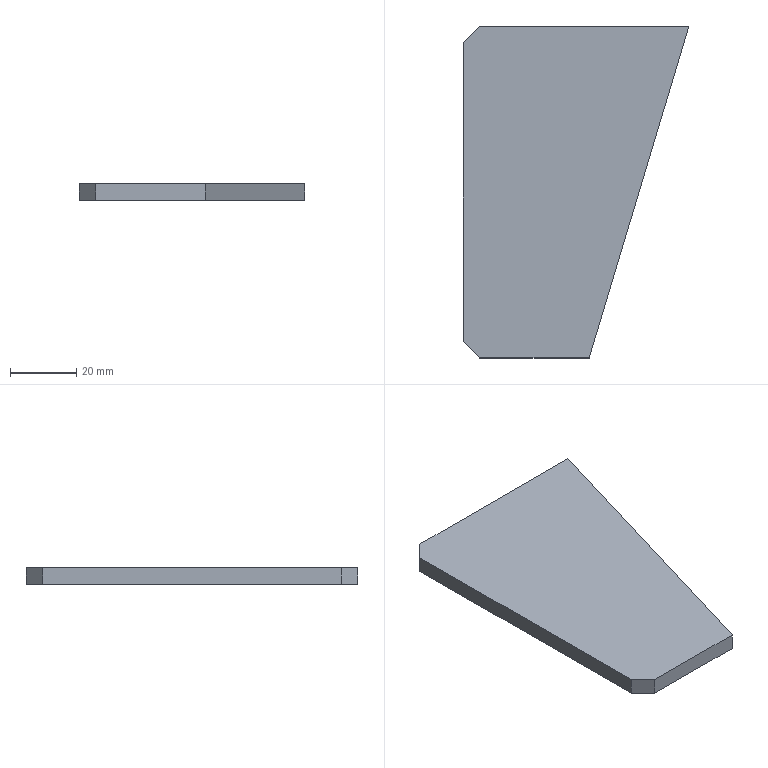Part | STEP file | 750038122 | 1 solid | 8 faces | box 68 x 100 x 5 mm | volume 26375 mm3 | plane 8
STEP:
#1=CARTESIAN_POINT('',(38.,0.,5.));
#2=VERTEX_POINT('',#1);
#3=CARTESIAN_POINT('',(5.,0.,5.));
#4=VERTEX_POINT('',#3);
#5=CARTESIAN_POINT('',(0.,0.,5.));
#6=DIRECTION('',(-1.,0.,0.));
#7=VECTOR('',#6,1000.);
#8=LINE('',#5,#7);
#9=EDGE_CURVE('',#2,#4,#8,.T.);
#10=ORIENTED_EDGE('',*,*,#9,.F.);
#11=CARTESIAN_POINT('',(68.,100.,5.));
#12=VERTEX_POINT('',#11);
#13=CARTESIAN_POINT('',(68.,100.,5.));
#14=DIRECTION('',(-0.2873,-0.9578,0.));
#15=VECTOR('',#14,1000.);
#16=LINE('',#13,#15);
#17=EDGE_CURVE('',#12,#2,#16,.T.);
#18=ORIENTED_EDGE('',*,*,#17,.F.);
#19=CARTESIAN_POINT('',(5.,100.,5.));
#20=VERTEX_POINT('',#19);
#21=CARTESIAN_POINT('',(0.,100.,5.));
#22=DIRECTION('',(1.,0.,0.));
#23=VECTOR('',#22,1000.);
#24=LINE('',#21,#23);
#25=EDGE_CURVE('',#20,#12,#24,.T.);
#26=ORIENTED_EDGE('',*,*,#25,.F.);
#27=CARTESIAN_POINT('',(0.,95.,5.));
#28=VERTEX_POINT('',#27);
#29=CARTESIAN_POINT('',(0.,95.,5.));
#30=DIRECTION('',(0.7071,0.7071,0.));
#31=VECTOR('',#30,1000.);
#32=LINE('',#29,#31);
#33=EDGE_CURVE('',#28,#20,#32,.T.);
#34=ORIENTED_EDGE('',*,*,#33,.F.);
#35=CARTESIAN_POINT('',(0.,5.,5.));
#36=VERTEX_POINT('',#35);
#37=CARTESIAN_POINT('',(0.,0.,5.));
#38=DIRECTION('',(0.,1.,0.));
#39=VECTOR('',#38,1000.);
#40=LINE('',#37,#39);
#41=EDGE_CURVE('',#36,#28,#40,.T.);
#42=ORIENTED_EDGE('',*,*,#41,.F.);
#43=CARTESIAN_POINT('',(5.,0.,5.));
#44=DIRECTION('',(-0.7071,0.7071,0.));
#45=VECTOR('',#44,1000.);
#46=LINE('',#43,#45);
#47=EDGE_CURVE('',#4,#36,#46,.T.);
#48=ORIENTED_EDGE('',*,*,#47,.F.);
#49=EDGE_LOOP('',(#10,#18,#26,#34,#42,#48));
#50=FACE_OUTER_BOUND('',#49,.T.);
#51=CARTESIAN_POINT('',(0.,0.,5.));
#52=DIRECTION('',(0.,0.,-1.));
#53=DIRECTION('',(-1.,0.,0.));
#54=AXIS2_PLACEMENT_3D('',#51,#52,#53);
#55=PLANE('',#54);
#56=ADVANCED_FACE('',(#50),#55,.F.);
#57=ORIENTED_EDGE('',*,*,#47,.T.);
#58=CARTESIAN_POINT('',(0.,5.,0.));
#59=VERTEX_POINT('',#58);
#60=CARTESIAN_POINT('',(0.,5.,5.));
#61=DIRECTION('',(0.,0.,-1.));
#62=VECTOR('',#61,1000.);
#63=LINE('',#60,#62);
#64=EDGE_CURVE('',#36,#59,#63,.T.);
#65=ORIENTED_EDGE('',*,*,#64,.T.);
#66=CARTESIAN_POINT('',(5.,0.,0.));
#67=VERTEX_POINT('',#66);
#68=CARTESIAN_POINT('',(5.,0.,0.));
#69=DIRECTION('',(0.7071,-0.7071,0.));
#70=VECTOR('',#69,1000.);
#71=LINE('',#68,#70);
#72=EDGE_CURVE('',#59,#67,#71,.T.);
#73=ORIENTED_EDGE('',*,*,#72,.T.);
#74=CARTESIAN_POINT('',(5.,0.,5.));
#75=DIRECTION('',(0.,0.,1.));
#76=VECTOR('',#75,1000.);
#77=LINE('',#74,#76);
#78=EDGE_CURVE('',#67,#4,#77,.T.);
#79=ORIENTED_EDGE('',*,*,#78,.T.);
#80=EDGE_LOOP('',(#57,#65,#73,#79));
#81=FACE_OUTER_BOUND('',#80,.T.);
#82=CARTESIAN_POINT('',(5.,0.,5.));
#83=DIRECTION('',(-0.7071,-0.7071,0.));
#84=DIRECTION('',(0.7071,-0.7071,0.));
#85=AXIS2_PLACEMENT_3D('',#82,#83,#84);
#86=PLANE('',#85);
#87=ADVANCED_FACE('',(#81),#86,.T.);
#88=ORIENTED_EDGE('',*,*,#9,.T.);
#89=ORIENTED_EDGE('',*,*,#78,.F.);
#90=CARTESIAN_POINT('',(38.,0.,0.));
#91=VERTEX_POINT('',#90);
#92=CARTESIAN_POINT('',(38.,0.,0.));
#93=DIRECTION('',(1.,0.,0.));
#94=VECTOR('',#93,1000.);
#95=LINE('',#92,#94);
#96=EDGE_CURVE('',#67,#91,#95,.T.);
#97=ORIENTED_EDGE('',*,*,#96,.T.);
#98=CARTESIAN_POINT('',(38.,0.,5.));
#99=DIRECTION('',(0.,0.,1.));
#100=VECTOR('',#99,1000.);
#101=LINE('',#98,#100);
#102=EDGE_CURVE('',#91,#2,#101,.T.);
#103=ORIENTED_EDGE('',*,*,#102,.T.);
#104=EDGE_LOOP('',(#88,#89,#97,#103));
#105=FACE_OUTER_BOUND('',#104,.T.);
#106=CARTESIAN_POINT('',(38.,0.,5.));
#107=DIRECTION('',(0.,-1.,0.));
#108=DIRECTION('',(0.,0.,-1.));
#109=AXIS2_PLACEMENT_3D('',#106,#107,#108);
#110=PLANE('',#109);
#111=ADVANCED_FACE('',(#105),#110,.T.);
#112=ORIENTED_EDGE('',*,*,#17,.T.);
#113=ORIENTED_EDGE('',*,*,#102,.F.);
#114=CARTESIAN_POINT('',(68.,100.,0.));
#115=VERTEX_POINT('',#114);
#116=CARTESIAN_POINT('',(68.,100.,0.));
#117=DIRECTION('',(0.2873,0.9578,0.));
#118=VECTOR('',#117,1000.);
#119=LINE('',#116,#118);
#120=EDGE_CURVE('',#91,#115,#119,.T.);
#121=ORIENTED_EDGE('',*,*,#120,.T.);
#122=CARTESIAN_POINT('',(68.,100.,5.));
#123=DIRECTION('',(0.,0.,1.));
#124=VECTOR('',#123,1000.);
#125=LINE('',#122,#124);
#126=EDGE_CURVE('',#115,#12,#125,.T.);
#127=ORIENTED_EDGE('',*,*,#126,.T.);
#128=EDGE_LOOP('',(#112,#113,#121,#127));
#129=FACE_OUTER_BOUND('',#128,.T.);
#130=CARTESIAN_POINT('',(68.,100.,5.));
#131=DIRECTION('',(0.9578,-0.2873,0.));
#132=DIRECTION('',(0.2873,0.9578,0.));
#133=AXIS2_PLACEMENT_3D('',#130,#131,#132);
#134=PLANE('',#133);
#135=ADVANCED_FACE('',(#129),#134,.T.);
#136=ORIENTED_EDGE('',*,*,#25,.T.);
#137=ORIENTED_EDGE('',*,*,#126,.F.);
#138=CARTESIAN_POINT('',(5.,100.,0.));
#139=VERTEX_POINT('',#138);
#140=CARTESIAN_POINT('',(5.,100.,0.));
#141=DIRECTION('',(-1.,0.,0.));
#142=VECTOR('',#141,1000.);
#143=LINE('',#140,#142);
#144=EDGE_CURVE('',#115,#139,#143,.T.);
#145=ORIENTED_EDGE('',*,*,#144,.T.);
#146=CARTESIAN_POINT('',(5.,100.,5.));
#147=DIRECTION('',(0.,0.,1.));
#148=VECTOR('',#147,1000.);
#149=LINE('',#146,#148);
#150=EDGE_CURVE('',#139,#20,#149,.T.);
#151=ORIENTED_EDGE('',*,*,#150,.T.);
#152=EDGE_LOOP('',(#136,#137,#145,#151));
#153=FACE_OUTER_BOUND('',#152,.T.);
#154=CARTESIAN_POINT('',(5.,100.,5.));
#155=DIRECTION('',(0.,1.,0.));
#156=DIRECTION('',(0.,0.,1.));
#157=AXIS2_PLACEMENT_3D('',#154,#155,#156);
#158=PLANE('',#157);
#159=ADVANCED_FACE('',(#153),#158,.T.);
#160=ORIENTED_EDGE('',*,*,#33,.T.);
#161=ORIENTED_EDGE('',*,*,#150,.F.);
#162=CARTESIAN_POINT('',(0.,95.,0.));
#163=VERTEX_POINT('',#162);
#164=CARTESIAN_POINT('',(0.,95.,0.));
#165=DIRECTION('',(-0.7071,-0.7071,0.));
#166=VECTOR('',#165,1000.);
#167=LINE('',#164,#166);
#168=EDGE_CURVE('',#139,#163,#167,.T.);
#169=ORIENTED_EDGE('',*,*,#168,.T.);
#170=CARTESIAN_POINT('',(0.,95.,5.));
#171=DIRECTION('',(0.,0.,1.));
#172=VECTOR('',#171,1000.);
#173=LINE('',#170,#172);
#174=EDGE_CURVE('',#163,#28,#173,.T.);
#175=ORIENTED_EDGE('',*,*,#174,.T.);
#176=EDGE_LOOP('',(#160,#161,#169,#175));
#177=FACE_OUTER_BOUND('',#176,.T.);
#178=CARTESIAN_POINT('',(0.,95.,5.));
#179=DIRECTION('',(-0.7071,0.7071,0.));
#180=DIRECTION('',(-0.7071,-0.7071,0.));
#181=AXIS2_PLACEMENT_3D('',#178,#179,#180);
#182=PLANE('',#181);
#183=ADVANCED_FACE('',(#177),#182,.T.);
#184=ORIENTED_EDGE('',*,*,#41,.T.);
#185=ORIENTED_EDGE('',*,*,#174,.F.);
#186=CARTESIAN_POINT('',(0.,5.,0.));
#187=DIRECTION('',(0.,-1.,0.));
#188=VECTOR('',#187,1000.);
#189=LINE('',#186,#188);
#190=EDGE_CURVE('',#163,#59,#189,.T.);
#191=ORIENTED_EDGE('',*,*,#190,.T.);
#192=ORIENTED_EDGE('',*,*,#64,.F.);
#193=EDGE_LOOP('',(#184,#185,#191,#192));
#194=FACE_OUTER_BOUND('',#193,.T.);
#195=CARTESIAN_POINT('',(0.,5.,5.));
#196=DIRECTION('',(-1.,0.,0.));
#197=DIRECTION('',(0.,-1.,0.));
#198=AXIS2_PLACEMENT_3D('',#195,#196,#197);
#199=PLANE('',#198);
#200=ADVANCED_FACE('',(#194),#199,.T.);
#201=ORIENTED_EDGE('',*,*,#120,.F.);
#202=ORIENTED_EDGE('',*,*,#96,.F.);
#203=ORIENTED_EDGE('',*,*,#72,.F.);
#204=ORIENTED_EDGE('',*,*,#190,.F.);
#205=ORIENTED_EDGE('',*,*,#168,.F.);
#206=ORIENTED_EDGE('',*,*,#144,.F.);
#207=EDGE_LOOP('',(#201,#202,#203,#204,#205,#206));
#208=FACE_OUTER_BOUND('',#207,.T.);
#209=CARTESIAN_POINT('',(0.,0.,0.));
#210=DIRECTION('',(0.,0.,-1.));
#211=DIRECTION('',(-1.,0.,0.));
#212=AXIS2_PLACEMENT_3D('',#209,#210,#211);
#213=PLANE('',#212);
#214=ADVANCED_FACE('',(#208),#213,.T.);
#215=CLOSED_SHELL('',(#56,#87,#111,#135,#159,#183,#200,#214));
#216=MANIFOLD_SOLID_BREP('',#215);
#217=CARTESIAN_POINT('',(0.,0.,0.));
#218=DIRECTION('',(0.,0.,1.));
#219=DIRECTION('',(1.,0.,0.));
#220=AXIS2_PLACEMENT_3D('',#217,#218,#219);
#221=(LENGTH_UNIT()NAMED_UNIT(*)SI_UNIT(.MILLI.,.METRE.));
#222=UNCERTAINTY_MEASURE_WITH_UNIT(LENGTH_MEASURE(0.00001),#221,'','');
#223=(NAMED_UNIT(*)PLANE_ANGLE_UNIT()SI_UNIT($,.RADIAN.));
#224=(NAMED_UNIT(*)SI_UNIT($,.STERADIAN.)SOLID_ANGLE_UNIT());
#225=(GEOMETRIC_REPRESENTATION_CONTEXT(3)GLOBAL_UNCERTAINTY_ASSIGNED_CONTEXT((#222))GLOBAL_UNIT_ASSIGNED_CONTEXT((#221,#223,#224))REPRESENTATION_CONTEXT('',''));
#226=ADVANCED_BREP_SHAPE_REPRESENTATION('',(#216,#220),#225);